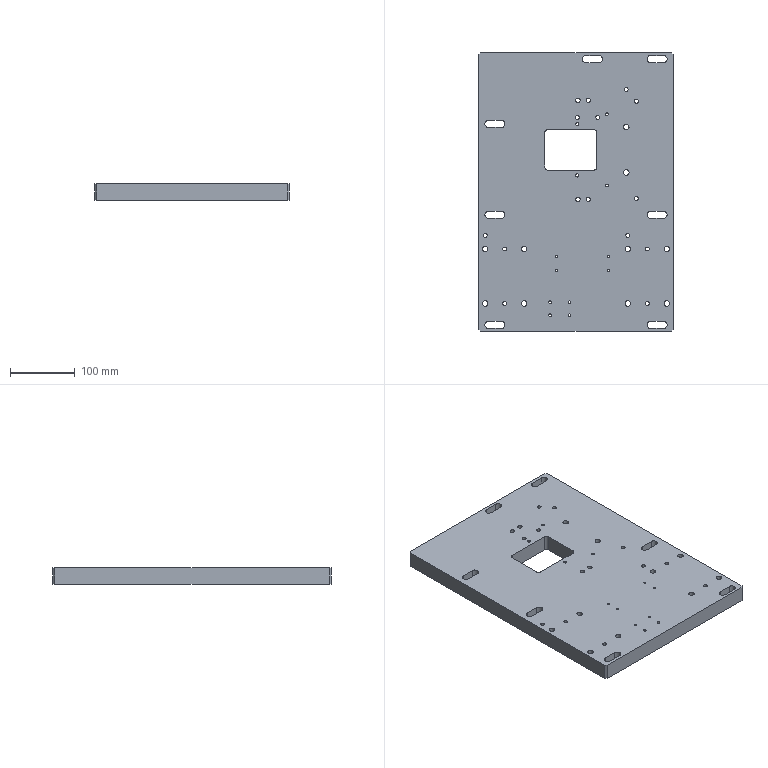Part | 1 solid | 83 faces | box 300 x 430 x 25 mm | volume 3014447 mm3 | cylinder 55 | plane 28 | commonest cylinder face diameters 11 x14 6 x11 8.5 x10 4.2 x6 3.3 x4 6.8 x4